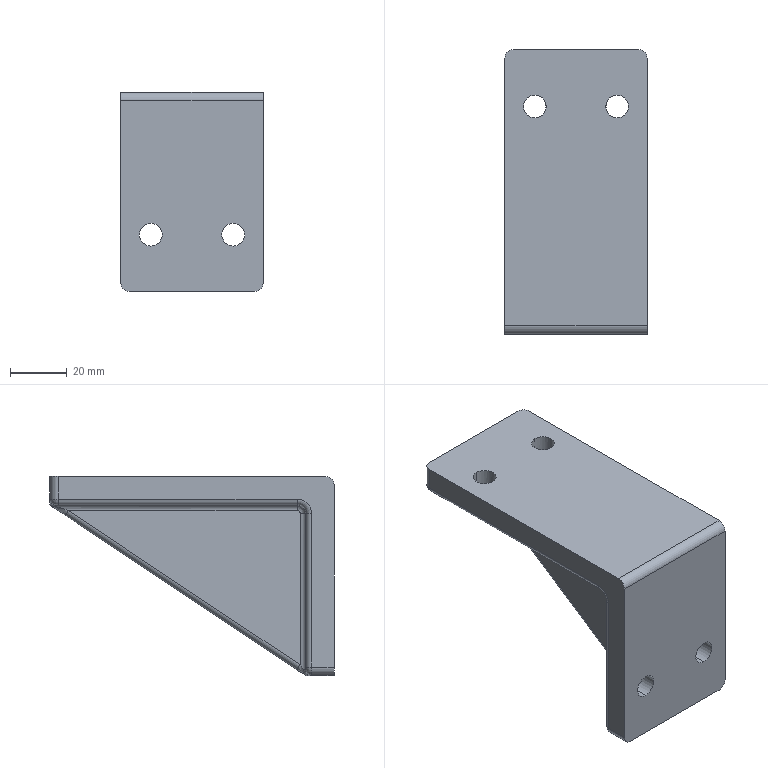Part | SolidWorks | features Fillet 5, ICE 3, MirrorPattern 2, Chamfer 1, Extrusion 1 | 1 solid | 66 faces | box 50 x 100 x 70 mm | volume 99196 mm3 | cylinder 29 | plane 13 | torus 12 | cone 8 | spline 4 | commonest cylinder face diameters 4 x14 8 x8 6 x7